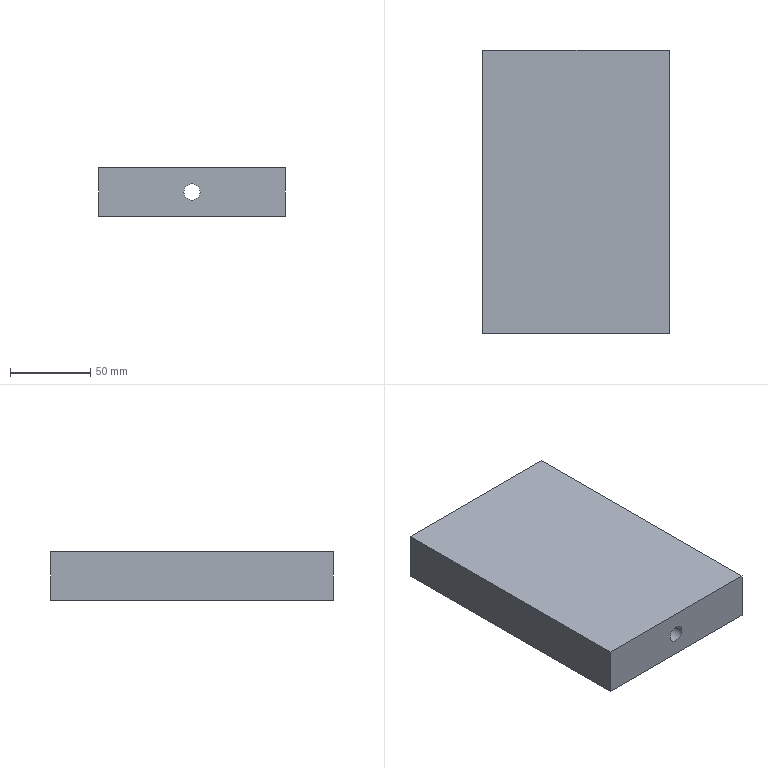Part | SolidWorks | features Extrusion 1, ICE 1 | 1 solid | 8 faces | box 116 x 176 x 30 mm | volume 598351 mm3 | plane 6 | cylinder 2 | commonest cylinder face diameters 10.11 x2
STEP:
#1=CARTESIAN_POINT('',(5.055,-88.,15.));
#2=VERTEX_POINT('',#1);
#3=CARTESIAN_POINT('',(-5.055,-88.,15.));
#4=VERTEX_POINT('',#3);
#5=CARTESIAN_POINT('',(0.,-88.,15.));
#6=DIRECTION('',(0.,1.,0.));
#7=DIRECTION('',(-1.,0.,0.));
#8=AXIS2_PLACEMENT_3D('',#5,#6,#7);
#9=CIRCLE('',#8,5.055);
#10=EDGE_CURVE('',#2,#4,#9,.T.);
#11=ORIENTED_EDGE('',*,*,#10,.F.);
#12=CARTESIAN_POINT('',(5.055,88.,15.));
#13=VERTEX_POINT('',#12);
#14=CARTESIAN_POINT('',(5.055,-88.,15.));
#15=DIRECTION('',(0.,1.,0.));
#16=VECTOR('',#15,1000.);
#17=LINE('',#14,#16);
#18=EDGE_CURVE('',#2,#13,#17,.T.);
#19=ORIENTED_EDGE('',*,*,#18,.T.);
#20=CARTESIAN_POINT('',(-5.055,88.,15.));
#21=VERTEX_POINT('',#20);
#22=CARTESIAN_POINT('',(0.,88.,15.));
#23=DIRECTION('',(0.,1.,0.));
#24=DIRECTION('',(-1.,0.,0.));
#25=AXIS2_PLACEMENT_3D('',#22,#23,#24);
#26=CIRCLE('',#25,5.055);
#27=EDGE_CURVE('',#13,#21,#26,.T.);
#28=ORIENTED_EDGE('',*,*,#27,.T.);
#29=CARTESIAN_POINT('',(-5.055,-88.,15.));
#30=DIRECTION('',(0.,1.,0.));
#31=VECTOR('',#30,1000.);
#32=LINE('',#29,#31);
#33=EDGE_CURVE('',#4,#21,#32,.T.);
#34=ORIENTED_EDGE('',*,*,#33,.F.);
#35=EDGE_LOOP('',(#11,#19,#28,#34));
#36=FACE_OUTER_BOUND('',#35,.T.);
#37=CARTESIAN_POINT('',(0.,-88.,15.));
#38=DIRECTION('',(0.,1.,0.));
#39=DIRECTION('',(-1.,0.,0.));
#40=AXIS2_PLACEMENT_3D('',#37,#38,#39);
#41=CYLINDRICAL_SURFACE('',#40,5.055);
#42=ADVANCED_FACE('',(#36),#41,.F.);
#43=CARTESIAN_POINT('',(-58.,88.,0.));
#44=VERTEX_POINT('',#43);
#45=CARTESIAN_POINT('',(-58.,-88.,0.));
#46=VERTEX_POINT('',#45);
#47=CARTESIAN_POINT('',(-58.,88.,0.));
#48=DIRECTION('',(0.,-1.,0.));
#49=VECTOR('',#48,1000.);
#50=LINE('',#47,#49);
#51=EDGE_CURVE('',#44,#46,#50,.T.);
#52=ORIENTED_EDGE('',*,*,#51,.T.);
#53=CARTESIAN_POINT('',(-58.,-88.,30.));
#54=VERTEX_POINT('',#53);
#55=CARTESIAN_POINT('',(-58.,-88.,30.));
#56=DIRECTION('',(0.,0.,-1.));
#57=VECTOR('',#56,1000.);
#58=LINE('',#55,#57);
#59=EDGE_CURVE('',#54,#46,#58,.T.);
#60=ORIENTED_EDGE('',*,*,#59,.F.);
#61=CARTESIAN_POINT('',(-58.,88.,30.));
#62=VERTEX_POINT('',#61);
#63=CARTESIAN_POINT('',(-58.,88.,30.));
#64=DIRECTION('',(0.,-1.,0.));
#65=VECTOR('',#64,1000.);
#66=LINE('',#63,#65);
#67=EDGE_CURVE('',#62,#54,#66,.T.);
#68=ORIENTED_EDGE('',*,*,#67,.F.);
#69=CARTESIAN_POINT('',(-58.,88.,30.));
#70=DIRECTION('',(0.,0.,-1.));
#71=VECTOR('',#70,1000.);
#72=LINE('',#69,#71);
#73=EDGE_CURVE('',#62,#44,#72,.T.);
#74=ORIENTED_EDGE('',*,*,#73,.T.);
#75=EDGE_LOOP('',(#52,#60,#68,#74));
#76=FACE_OUTER_BOUND('',#75,.T.);
#77=CARTESIAN_POINT('',(-58.,88.,30.));
#78=DIRECTION('',(1.,0.,0.));
#79=DIRECTION('',(0.,1.,0.));
#80=AXIS2_PLACEMENT_3D('',#77,#78,#79);
#81=PLANE('',#80);
#82=ADVANCED_FACE('',(#76),#81,.F.);
#83=CARTESIAN_POINT('',(0.,-88.,15.));
#84=DIRECTION('',(0.,1.,0.));
#85=DIRECTION('',(-1.,0.,0.));
#86=AXIS2_PLACEMENT_3D('',#83,#84,#85);
#87=CIRCLE('',#86,5.055);
#88=EDGE_CURVE('',#4,#2,#87,.T.);
#89=ORIENTED_EDGE('',*,*,#88,.T.);
#90=ORIENTED_EDGE('',*,*,#10,.T.);
#91=EDGE_LOOP('',(#89,#90));
#92=FACE_BOUND('',#91,.T.);
#93=CARTESIAN_POINT('',(58.,-88.,0.));
#94=VERTEX_POINT('',#93);
#95=CARTESIAN_POINT('',(58.,-88.,0.));
#96=DIRECTION('',(1.,0.,0.));
#97=VECTOR('',#96,1000.);
#98=LINE('',#95,#97);
#99=EDGE_CURVE('',#46,#94,#98,.T.);
#100=ORIENTED_EDGE('',*,*,#99,.T.);
#101=CARTESIAN_POINT('',(58.,-88.,30.));
#102=VERTEX_POINT('',#101);
#103=CARTESIAN_POINT('',(58.,-88.,30.));
#104=DIRECTION('',(0.,0.,-1.));
#105=VECTOR('',#104,1000.);
#106=LINE('',#103,#105);
#107=EDGE_CURVE('',#102,#94,#106,.T.);
#108=ORIENTED_EDGE('',*,*,#107,.F.);
#109=CARTESIAN_POINT('',(58.,-88.,30.));
#110=DIRECTION('',(1.,0.,0.));
#111=VECTOR('',#110,1000.);
#112=LINE('',#109,#111);
#113=EDGE_CURVE('',#54,#102,#112,.T.);
#114=ORIENTED_EDGE('',*,*,#113,.F.);
#115=ORIENTED_EDGE('',*,*,#59,.T.);
#116=EDGE_LOOP('',(#100,#108,#114,#115));
#117=FACE_OUTER_BOUND('',#116,.T.);
#118=CARTESIAN_POINT('',(58.,-88.,30.));
#119=DIRECTION('',(0.,1.,0.));
#120=DIRECTION('',(-1.,0.,0.));
#121=AXIS2_PLACEMENT_3D('',#118,#119,#120);
#122=PLANE('',#121);
#123=ADVANCED_FACE('',(#92,#117),#122,.F.);
#124=CARTESIAN_POINT('',(58.,88.,0.));
#125=VERTEX_POINT('',#124);
#126=CARTESIAN_POINT('',(58.,88.,0.));
#127=DIRECTION('',(0.,1.,0.));
#128=VECTOR('',#127,1000.);
#129=LINE('',#126,#128);
#130=EDGE_CURVE('',#94,#125,#129,.T.);
#131=ORIENTED_EDGE('',*,*,#130,.T.);
#132=CARTESIAN_POINT('',(58.,88.,30.));
#133=VERTEX_POINT('',#132);
#134=CARTESIAN_POINT('',(58.,88.,30.));
#135=DIRECTION('',(0.,0.,-1.));
#136=VECTOR('',#135,1000.);
#137=LINE('',#134,#136);
#138=EDGE_CURVE('',#133,#125,#137,.T.);
#139=ORIENTED_EDGE('',*,*,#138,.F.);
#140=CARTESIAN_POINT('',(58.,88.,30.));
#141=DIRECTION('',(0.,1.,0.));
#142=VECTOR('',#141,1000.);
#143=LINE('',#140,#142);
#144=EDGE_CURVE('',#102,#133,#143,.T.);
#145=ORIENTED_EDGE('',*,*,#144,.F.);
#146=ORIENTED_EDGE('',*,*,#107,.T.);
#147=EDGE_LOOP('',(#131,#139,#145,#146));
#148=FACE_OUTER_BOUND('',#147,.T.);
#149=CARTESIAN_POINT('',(58.,88.,30.));
#150=DIRECTION('',(-1.,0.,0.));
#151=DIRECTION('',(0.,-1.,0.));
#152=AXIS2_PLACEMENT_3D('',#149,#150,#151);
#153=PLANE('',#152);
#154=ADVANCED_FACE('',(#148),#153,.F.);
#155=CARTESIAN_POINT('',(0.,88.,15.));
#156=DIRECTION('',(0.,1.,0.));
#157=DIRECTION('',(-1.,0.,0.));
#158=AXIS2_PLACEMENT_3D('',#155,#156,#157);
#159=CIRCLE('',#158,5.055);
#160=EDGE_CURVE('',#21,#13,#159,.T.);
#161=ORIENTED_EDGE('',*,*,#160,.F.);
#162=ORIENTED_EDGE('',*,*,#27,.F.);
#163=EDGE_LOOP('',(#161,#162));
#164=FACE_BOUND('',#163,.T.);
#165=CARTESIAN_POINT('',(58.,88.,0.));
#166=DIRECTION('',(-1.,0.,0.));
#167=VECTOR('',#166,1000.);
#168=LINE('',#165,#167);
#169=EDGE_CURVE('',#125,#44,#168,.T.);
#170=ORIENTED_EDGE('',*,*,#169,.T.);
#171=ORIENTED_EDGE('',*,*,#73,.F.);
#172=CARTESIAN_POINT('',(58.,88.,30.));
#173=DIRECTION('',(-1.,0.,0.));
#174=VECTOR('',#173,1000.);
#175=LINE('',#172,#174);
#176=EDGE_CURVE('',#133,#62,#175,.T.);
#177=ORIENTED_EDGE('',*,*,#176,.F.);
#178=ORIENTED_EDGE('',*,*,#138,.T.);
#179=EDGE_LOOP('',(#170,#171,#177,#178));
#180=FACE_OUTER_BOUND('',#179,.T.);
#181=CARTESIAN_POINT('',(58.,88.,30.));
#182=DIRECTION('',(0.,-1.,0.));
#183=DIRECTION('',(1.,0.,0.));
#184=AXIS2_PLACEMENT_3D('',#181,#182,#183);
#185=PLANE('',#184);
#186=ADVANCED_FACE('',(#164,#180),#185,.F.);
#187=ORIENTED_EDGE('',*,*,#67,.T.);
#188=ORIENTED_EDGE('',*,*,#113,.T.);
#189=ORIENTED_EDGE('',*,*,#144,.T.);
#190=ORIENTED_EDGE('',*,*,#176,.T.);
#191=EDGE_LOOP('',(#187,#188,#189,#190));
#192=FACE_OUTER_BOUND('',#191,.T.);
#193=CARTESIAN_POINT('',(0.,0.,30.));
#194=DIRECTION('',(0.,0.,-1.));
#195=DIRECTION('',(-1.,0.,0.));
#196=AXIS2_PLACEMENT_3D('',#193,#194,#195);
#197=PLANE('',#196);
#198=ADVANCED_FACE('',(#192),#197,.F.);
#199=ORIENTED_EDGE('',*,*,#51,.F.);
#200=ORIENTED_EDGE('',*,*,#169,.F.);
#201=ORIENTED_EDGE('',*,*,#130,.F.);
#202=ORIENTED_EDGE('',*,*,#99,.F.);
#203=EDGE_LOOP('',(#199,#200,#201,#202));
#204=FACE_OUTER_BOUND('',#203,.T.);
#205=CARTESIAN_POINT('',(0.,0.,0.));
#206=DIRECTION('',(0.,0.,-1.));
#207=DIRECTION('',(-1.,0.,0.));
#208=AXIS2_PLACEMENT_3D('',#205,#206,#207);
#209=PLANE('',#208);
#210=ADVANCED_FACE('',(#204),#209,.T.);
#211=ORIENTED_EDGE('',*,*,#18,.F.);
#212=ORIENTED_EDGE('',*,*,#88,.F.);
#213=ORIENTED_EDGE('',*,*,#33,.T.);
#214=ORIENTED_EDGE('',*,*,#160,.T.);
#215=EDGE_LOOP('',(#211,#212,#213,#214));
#216=FACE_OUTER_BOUND('',#215,.T.);
#217=CARTESIAN_POINT('',(0.,-88.,15.));
#218=DIRECTION('',(0.,1.,0.));
#219=DIRECTION('',(-1.,0.,0.));
#220=AXIS2_PLACEMENT_3D('',#217,#218,#219);
#221=CYLINDRICAL_SURFACE('',#220,5.055);
#222=ADVANCED_FACE('',(#216),#221,.F.);
#223=CLOSED_SHELL('',(#42,#82,#123,#154,#186,#198,#210,#222));
#224=MANIFOLD_SOLID_BREP('',#223);
#225=CARTESIAN_POINT('',(0.,0.,0.));
#226=DIRECTION('',(0.,0.,1.));
#227=DIRECTION('',(1.,0.,0.));
#228=AXIS2_PLACEMENT_3D('',#225,#226,#227);
#229=(LENGTH_UNIT()NAMED_UNIT(*)SI_UNIT(.MILLI.,.METRE.));
#230=UNCERTAINTY_MEASURE_WITH_UNIT(LENGTH_MEASURE(0.00001),#229,'','');
#231=(NAMED_UNIT(*)PLANE_ANGLE_UNIT()SI_UNIT($,.RADIAN.));
#232=(NAMED_UNIT(*)SI_UNIT($,.STERADIAN.)SOLID_ANGLE_UNIT());
#233=(GEOMETRIC_REPRESENTATION_CONTEXT(3)GLOBAL_UNCERTAINTY_ASSIGNED_CONTEXT((#230))GLOBAL_UNIT_ASSIGNED_CONTEXT((#229,#231,#232))REPRESENTATION_CONTEXT('',''));
#234=ADVANCED_BREP_SHAPE_REPRESENTATION('',(#224,#228),#233);